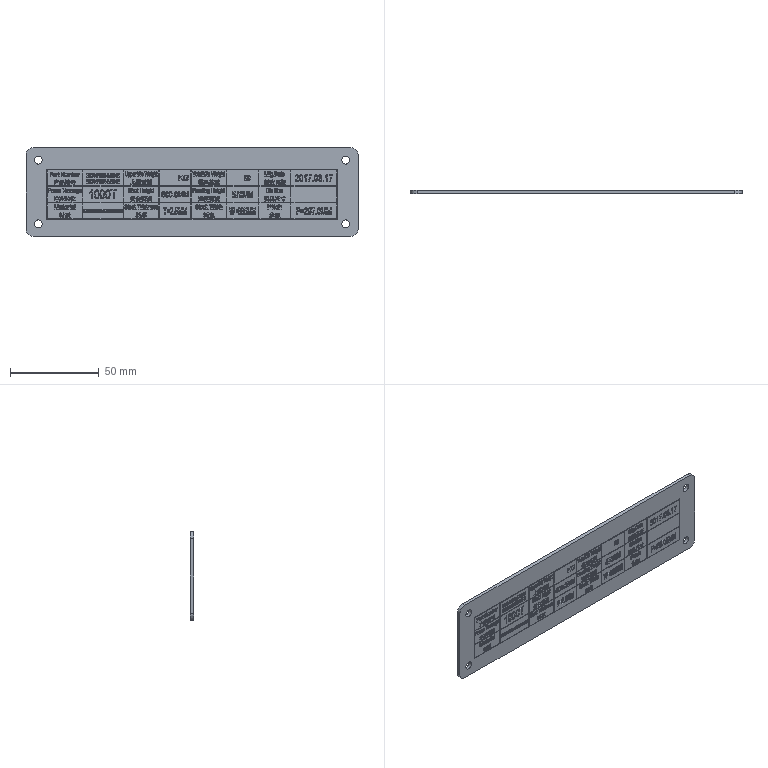Part | STEP file | lll_id3730_x_t | 1 solid | 4496 faces | volume 18390 mm3 | plane 2736 | other 1703 | cylinder 57 | commonest cylinder face diameters 4.5 x4 8 x4 1.374 x2 1.941 x2 2.036 x2 2.285 x2